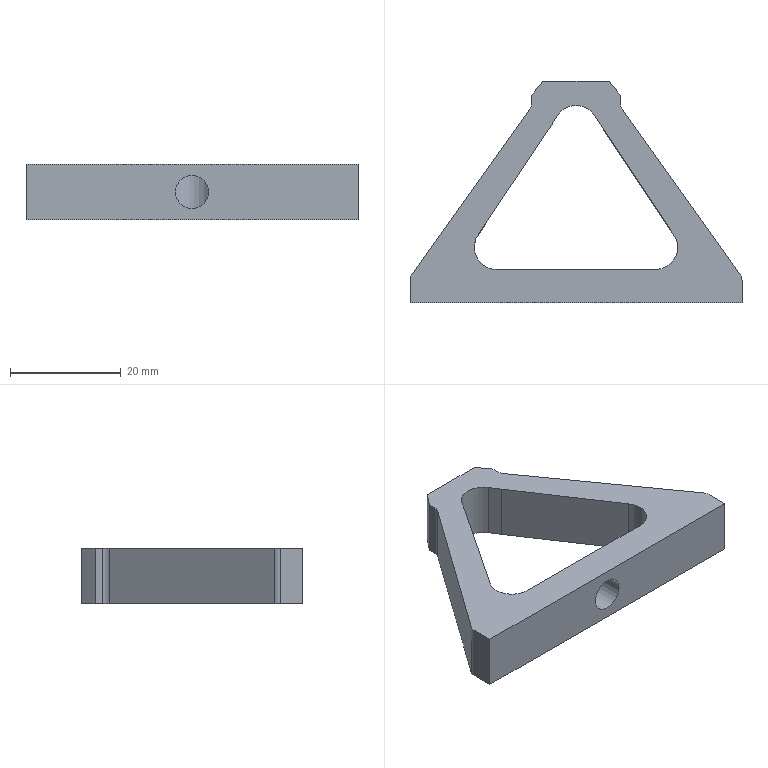Part | SolidWorks | features Extrusion 1, ICE 1 | 1 solid | 27 faces | box 60 x 40 x 10 mm | volume 8175 mm3 | plane 17 | cylinder 10 | commonest cylinder face diameters 4 x4 8 x4 6 x2
STEP:
#1=CARTESIAN_POINT('',(-3.485,-13.953,5.));
#2=VERTEX_POINT('',#1);
#3=CARTESIAN_POINT('',(-9.485,-13.953,5.));
#4=VERTEX_POINT('',#3);
#5=CARTESIAN_POINT('',(-6.485,-13.953,5.));
#6=DIRECTION('',(0.,1.,0.));
#7=DIRECTION('',(-1.,0.,0.));
#8=AXIS2_PLACEMENT_3D('',#5,#6,#7);
#9=CIRCLE('',#8,3.);
#10=EDGE_CURVE('',#2,#4,#9,.T.);
#11=ORIENTED_EDGE('',*,*,#10,.T.);
#12=CARTESIAN_POINT('',(-9.485,-19.953,5.));
#13=VERTEX_POINT('',#12);
#14=CARTESIAN_POINT('',(-9.485,-9.953,5.));
#15=DIRECTION('',(0.,-1.,0.));
#16=VECTOR('',#15,1000.);
#17=LINE('',#14,#16);
#18=EDGE_CURVE('',#4,#13,#17,.T.);
#19=ORIENTED_EDGE('',*,*,#18,.T.);
#20=CARTESIAN_POINT('',(-3.485,-19.953,5.));
#21=VERTEX_POINT('',#20);
#22=CARTESIAN_POINT('',(-6.485,-19.953,5.));
#23=DIRECTION('',(0.,-1.,0.));
#24=DIRECTION('',(1.,0.,0.));
#25=AXIS2_PLACEMENT_3D('',#22,#23,#24);
#26=CIRCLE('',#25,3.);
#27=EDGE_CURVE('',#13,#21,#26,.T.);
#28=ORIENTED_EDGE('',*,*,#27,.T.);
#29=CARTESIAN_POINT('',(-3.485,-9.953,5.));
#30=DIRECTION('',(0.,-1.,0.));
#31=VECTOR('',#30,1000.);
#32=LINE('',#29,#31);
#33=EDGE_CURVE('',#2,#21,#32,.T.);
#34=ORIENTED_EDGE('',*,*,#33,.F.);
#35=EDGE_LOOP('',(#11,#19,#28,#34));
#36=FACE_OUTER_BOUND('',#35,.T.);
#37=CARTESIAN_POINT('',(-6.485,-9.953,5.));
#38=DIRECTION('',(0.,-1.,0.));
#39=DIRECTION('',(1.,0.,0.));
#40=AXIS2_PLACEMENT_3D('',#37,#38,#39);
#41=CYLINDRICAL_SURFACE('',#40,3.);
#42=ADVANCED_FACE('',(#36),#41,.F.);
#43=CARTESIAN_POINT('',(-24.192,-7.733,10.));
#44=VERTEX_POINT('',#43);
#45=CARTESIAN_POINT('',(-24.865,-9.953,10.));
#46=VERTEX_POINT('',#45);
#47=CARTESIAN_POINT('',(-20.865,-9.953,10.));
#48=DIRECTION('',(0.,0.,1.));
#49=DIRECTION('',(-1.,0.,0.));
#50=AXIS2_PLACEMENT_3D('',#47,#48,#49);
#51=CIRCLE('',#50,4.);
#52=EDGE_CURVE('',#44,#46,#51,.T.);
#53=ORIENTED_EDGE('',*,*,#52,.T.);
#54=CARTESIAN_POINT('',(-24.865,-9.953,0.));
#55=VERTEX_POINT('',#54);
#56=CARTESIAN_POINT('',(-24.865,-9.953,10.));
#57=DIRECTION('',(0.,0.,-1.));
#58=VECTOR('',#57,1000.);
#59=LINE('',#56,#58);
#60=EDGE_CURVE('',#46,#55,#59,.T.);
#61=ORIENTED_EDGE('',*,*,#60,.T.);
#62=CARTESIAN_POINT('',(-24.192,-7.733,0.));
#63=VERTEX_POINT('',#62);
#64=CARTESIAN_POINT('',(-20.865,-9.953,0.));
#65=DIRECTION('',(0.,0.,1.));
#66=DIRECTION('',(-1.,0.,0.));
#67=AXIS2_PLACEMENT_3D('',#64,#65,#66);
#68=CIRCLE('',#67,4.);
#69=EDGE_CURVE('',#63,#55,#68,.T.);
#70=ORIENTED_EDGE('',*,*,#69,.F.);
#71=CARTESIAN_POINT('',(-24.192,-7.733,10.));
#72=DIRECTION('',(0.,0.,-1.));
#73=VECTOR('',#72,1000.);
#74=LINE('',#71,#73);
#75=EDGE_CURVE('',#44,#63,#74,.T.);
#76=ORIENTED_EDGE('',*,*,#75,.F.);
#77=EDGE_LOOP('',(#53,#61,#70,#76));
#78=FACE_OUTER_BOUND('',#77,.T.);
#79=CARTESIAN_POINT('',(-20.865,-9.953,10.));
#80=DIRECTION('',(0.,0.,-1.));
#81=DIRECTION('',(-1.,0.,0.));
#82=AXIS2_PLACEMENT_3D('',#79,#80,#81);
#83=CYLINDRICAL_SURFACE('',#82,4.);
#84=ADVANCED_FACE('',(#78),#83,.F.);
#85=CARTESIAN_POINT('',(-36.485,-15.953,10.));
#86=VERTEX_POINT('',#85);
#87=CARTESIAN_POINT('',(-36.485,-19.953,10.));
#88=VERTEX_POINT('',#87);
#89=CARTESIAN_POINT('',(-36.485,-19.953,10.));
#90=DIRECTION('',(0.,-1.,0.));
#91=VECTOR('',#90,1000.);
#92=LINE('',#89,#91);
#93=EDGE_CURVE('',#86,#88,#92,.T.);
#94=ORIENTED_EDGE('',*,*,#93,.T.);
#95=CARTESIAN_POINT('',(23.515,-19.953,10.));
#96=VERTEX_POINT('',#95);
#97=CARTESIAN_POINT('',(-36.485,-19.953,10.));
#98=DIRECTION('',(1.,0.,0.));
#99=VECTOR('',#98,1000.);
#100=LINE('',#97,#99);
#101=EDGE_CURVE('',#88,#96,#100,.T.);
#102=ORIENTED_EDGE('',*,*,#101,.T.);
#103=CARTESIAN_POINT('',(23.515,-15.953,10.));
#104=VERTEX_POINT('',#103);
#105=CARTESIAN_POINT('',(23.515,-19.953,10.));
#106=DIRECTION('',(0.,1.,0.));
#107=VECTOR('',#106,1000.);
#108=LINE('',#105,#107);
#109=EDGE_CURVE('',#96,#104,#108,.T.);
#110=ORIENTED_EDGE('',*,*,#109,.T.);
#111=CARTESIAN_POINT('',(23.179,-14.843,10.));
#112=VERTEX_POINT('',#111);
#113=CARTESIAN_POINT('',(21.515,-15.953,10.));
#114=DIRECTION('',(0.,0.,1.));
#115=DIRECTION('',(1.,0.,0.));
#116=AXIS2_PLACEMENT_3D('',#113,#114,#115);
#117=CIRCLE('',#116,2.);
#118=EDGE_CURVE('',#104,#112,#117,.T.);
#119=ORIENTED_EDGE('',*,*,#118,.T.);
#120=CARTESIAN_POINT('',(1.887,15.02,10.));
#121=VERTEX_POINT('',#120);
#122=CARTESIAN_POINT('',(1.887,15.02,10.));
#123=DIRECTION('',(-0.5805,0.8142,0.));
#124=VECTOR('',#123,1000.);
#125=LINE('',#122,#124);
#126=EDGE_CURVE('',#112,#121,#125,.T.);
#127=ORIENTED_EDGE('',*,*,#126,.T.);
#128=CARTESIAN_POINT('',(1.515,16.181,10.));
#129=VERTEX_POINT('',#128);
#130=CARTESIAN_POINT('',(3.515,16.181,10.));
#131=DIRECTION('',(0.,0.,-1.));
#132=DIRECTION('',(-1.,0.,0.));
#133=AXIS2_PLACEMENT_3D('',#130,#131,#132);
#134=CIRCLE('',#133,2.);
#135=EDGE_CURVE('',#121,#129,#134,.T.);
#136=ORIENTED_EDGE('',*,*,#135,.T.);
#137=CARTESIAN_POINT('',(1.515,17.541,10.));
#138=VERTEX_POINT('',#137);
#139=CARTESIAN_POINT('',(1.515,16.181,10.));
#140=DIRECTION('',(0.,1.,0.));
#141=VECTOR('',#140,1000.);
#142=LINE('',#139,#141);
#143=EDGE_CURVE('',#129,#138,#142,.T.);
#144=ORIENTED_EDGE('',*,*,#143,.T.);
#145=CARTESIAN_POINT('',(-0.4847,20.047,10.));
#146=VERTEX_POINT('',#145);
#147=CARTESIAN_POINT('',(1.515,17.541,10.));
#148=DIRECTION('',(-0.6238,0.7816,0.));
#149=VECTOR('',#148,1000.);
#150=LINE('',#147,#149);
#151=EDGE_CURVE('',#138,#146,#150,.T.);
#152=ORIENTED_EDGE('',*,*,#151,.T.);
#153=CARTESIAN_POINT('',(-12.485,20.047,10.));
#154=VERTEX_POINT('',#153);
#155=CARTESIAN_POINT('',(-12.485,20.047,10.));
#156=DIRECTION('',(-1.,0.,0.));
#157=VECTOR('',#156,1000.);
#158=LINE('',#155,#157);
#159=EDGE_CURVE('',#146,#154,#158,.T.);
#160=ORIENTED_EDGE('',*,*,#159,.T.);
#161=CARTESIAN_POINT('',(-14.485,17.541,10.));
#162=VERTEX_POINT('',#161);
#163=CARTESIAN_POINT('',(-14.485,17.541,10.));
#164=DIRECTION('',(-0.6238,-0.7816,0.));
#165=VECTOR('',#164,1000.);
#166=LINE('',#163,#165);
#167=EDGE_CURVE('',#154,#162,#166,.T.);
#168=ORIENTED_EDGE('',*,*,#167,.T.);
#169=CARTESIAN_POINT('',(-14.485,16.181,10.));
#170=VERTEX_POINT('',#169);
#171=CARTESIAN_POINT('',(-14.485,16.181,10.));
#172=DIRECTION('',(0.,-1.,0.));
#173=VECTOR('',#172,1000.);
#174=LINE('',#171,#173);
#175=EDGE_CURVE('',#162,#170,#174,.T.);
#176=ORIENTED_EDGE('',*,*,#175,.T.);
#177=CARTESIAN_POINT('',(-14.856,15.02,10.));
#178=VERTEX_POINT('',#177);
#179=CARTESIAN_POINT('',(-16.485,16.181,10.));
#180=DIRECTION('',(0.,0.,-1.));
#181=DIRECTION('',(1.,0.,0.));
#182=AXIS2_PLACEMENT_3D('',#179,#180,#181);
#183=CIRCLE('',#182,2.);
#184=EDGE_CURVE('',#170,#178,#183,.T.);
#185=ORIENTED_EDGE('',*,*,#184,.T.);
#186=CARTESIAN_POINT('',(-36.148,-14.843,10.));
#187=VERTEX_POINT('',#186);
#188=CARTESIAN_POINT('',(-36.148,-14.843,10.));
#189=DIRECTION('',(-0.5805,-0.8142,0.));
#190=VECTOR('',#189,1000.);
#191=LINE('',#188,#190);
#192=EDGE_CURVE('',#178,#187,#191,.T.);
#193=ORIENTED_EDGE('',*,*,#192,.T.);
#194=CARTESIAN_POINT('',(-34.485,-15.953,10.));
#195=DIRECTION('',(0.,0.,1.));
#196=DIRECTION('',(-1.,0.,0.));
#197=AXIS2_PLACEMENT_3D('',#194,#195,#196);
#198=CIRCLE('',#197,2.);
#199=EDGE_CURVE('',#187,#86,#198,.T.);
#200=ORIENTED_EDGE('',*,*,#199,.T.);
#201=EDGE_LOOP('',(#94,#102,#110,#119,#127,#136,#144,#152,#160,#168,#176,#185,#193,#200));
#202=FACE_OUTER_BOUND('',#201,.T.);
#203=CARTESIAN_POINT('',(-9.853,13.848,10.));
#204=VERTEX_POINT('',#203);
#205=CARTESIAN_POINT('',(-11.182,11.768,10.));
#206=VERTEX_POINT('',#205);
#207=CARTESIAN_POINT('',(-11.182,11.768,10.));
#208=DIRECTION('',(-0.5383,-0.8427,0.));
#209=VECTOR('',#208,1000.);
#210=LINE('',#207,#209);
#211=EDGE_CURVE('',#204,#206,#210,.T.);
#212=ORIENTED_EDGE('',*,*,#211,.F.);
#213=CARTESIAN_POINT('',(-3.113,13.85,10.));
#214=VERTEX_POINT('',#213);
#215=CARTESIAN_POINT('',(-6.482,11.695,10.));
#216=DIRECTION('',(0.,0.,1.));
#217=DIRECTION('',(1.,0.,0.));
#218=AXIS2_PLACEMENT_3D('',#215,#216,#217);
#219=CIRCLE('',#218,4.);
#220=EDGE_CURVE('',#214,#204,#219,.T.);
#221=ORIENTED_EDGE('',*,*,#220,.F.);
#222=CARTESIAN_POINT('',(-1.803,11.803,10.));
#223=VERTEX_POINT('',#222);
#224=CARTESIAN_POINT('',(-1.803,11.803,10.));
#225=DIRECTION('',(-0.5389,0.8424,0.));
#226=VECTOR('',#225,1000.);
#227=LINE('',#224,#226);
#228=EDGE_CURVE('',#223,#214,#227,.T.);
#229=ORIENTED_EDGE('',*,*,#228,.F.);
#230=CARTESIAN_POINT('',(11.226,-7.734,10.));
#231=VERTEX_POINT('',#230);
#232=CARTESIAN_POINT('',(-1.803,11.803,10.));
#233=DIRECTION('',(-0.5548,0.832,0.));
#234=VECTOR('',#233,1000.);
#235=LINE('',#232,#234);
#236=EDGE_CURVE('',#231,#223,#235,.T.);
#237=ORIENTED_EDGE('',*,*,#236,.F.);
#238=CARTESIAN_POINT('',(7.898,-13.953,10.));
#239=VERTEX_POINT('',#238);
#240=CARTESIAN_POINT('',(7.898,-9.953,10.));
#241=DIRECTION('',(0.,0.,1.));
#242=DIRECTION('',(-1.,0.,0.));
#243=AXIS2_PLACEMENT_3D('',#240,#241,#242);
#244=CIRCLE('',#243,4.);
#245=EDGE_CURVE('',#239,#231,#244,.T.);
#246=ORIENTED_EDGE('',*,*,#245,.F.);
#247=CARTESIAN_POINT('',(-20.865,-13.953,10.));
#248=VERTEX_POINT('',#247);
#249=CARTESIAN_POINT('',(-20.865,-13.953,10.));
#250=DIRECTION('',(1.,0.,0.));
#251=VECTOR('',#250,1000.);
#252=LINE('',#249,#251);
#253=EDGE_CURVE('',#248,#239,#252,.T.);
#254=ORIENTED_EDGE('',*,*,#253,.F.);
#255=CARTESIAN_POINT('',(-20.865,-9.953,10.));
#256=DIRECTION('',(0.,0.,1.));
#257=DIRECTION('',(-1.,0.,0.));
#258=AXIS2_PLACEMENT_3D('',#255,#256,#257);
#259=CIRCLE('',#258,4.);
#260=EDGE_CURVE('',#46,#248,#259,.T.);
#261=ORIENTED_EDGE('',*,*,#260,.F.);
#262=ORIENTED_EDGE('',*,*,#52,.F.);
#263=CARTESIAN_POINT('',(-24.192,-7.733,10.));
#264=DIRECTION('',(-0.555,-0.8319,0.));
#265=VECTOR('',#264,1000.);
#266=LINE('',#263,#265);
#267=EDGE_CURVE('',#206,#44,#266,.T.);
#268=ORIENTED_EDGE('',*,*,#267,.F.);
#269=EDGE_LOOP('',(#212,#221,#229,#237,#246,#254,#261,#262,#268));
#270=FACE_BOUND('',#269,.T.);
#271=CARTESIAN_POINT('',(-34.485,-15.953,10.));
#272=DIRECTION('',(0.,0.,-1.));
#273=DIRECTION('',(-1.,0.,0.));
#274=AXIS2_PLACEMENT_3D('',#271,#272,#273);
#275=PLANE('',#274);
#276=ADVANCED_FACE('',(#202,#270),#275,.F.);
#277=CARTESIAN_POINT('',(-36.485,-15.953,0.));
#278=VERTEX_POINT('',#277);
#279=CARTESIAN_POINT('',(-36.485,-19.953,0.));
#280=VERTEX_POINT('',#279);
#281=CARTESIAN_POINT('',(-36.485,-19.953,0.));
#282=DIRECTION('',(0.,-1.,0.));
#283=VECTOR('',#282,1000.);
#284=LINE('',#281,#283);
#285=EDGE_CURVE('',#278,#280,#284,.T.);
#286=ORIENTED_EDGE('',*,*,#285,.F.);
#287=CARTESIAN_POINT('',(-36.148,-14.843,0.));
#288=VERTEX_POINT('',#287);
#289=CARTESIAN_POINT('',(-34.485,-15.953,0.));
#290=DIRECTION('',(0.,0.,1.));
#291=DIRECTION('',(-1.,0.,0.));
#292=AXIS2_PLACEMENT_3D('',#289,#290,#291);
#293=CIRCLE('',#292,2.);
#294=EDGE_CURVE('',#288,#278,#293,.T.);
#295=ORIENTED_EDGE('',*,*,#294,.F.);
#296=CARTESIAN_POINT('',(-14.856,15.02,0.));
#297=VERTEX_POINT('',#296);
#298=CARTESIAN_POINT('',(-36.148,-14.843,0.));
#299=DIRECTION('',(-0.5805,-0.8142,0.));
#300=VECTOR('',#299,1000.);
#301=LINE('',#298,#300);
#302=EDGE_CURVE('',#297,#288,#301,.T.);
#303=ORIENTED_EDGE('',*,*,#302,.F.);
#304=CARTESIAN_POINT('',(-14.485,16.181,0.));
#305=VERTEX_POINT('',#304);
#306=CARTESIAN_POINT('',(-16.485,16.181,0.));
#307=DIRECTION('',(0.,0.,-1.));
#308=DIRECTION('',(1.,0.,0.));
#309=AXIS2_PLACEMENT_3D('',#306,#307,#308);
#310=CIRCLE('',#309,2.);
#311=EDGE_CURVE('',#305,#297,#310,.T.);
#312=ORIENTED_EDGE('',*,*,#311,.F.);
#313=CARTESIAN_POINT('',(-14.485,17.541,0.));
#314=VERTEX_POINT('',#313);
#315=CARTESIAN_POINT('',(-14.485,16.181,0.));
#316=DIRECTION('',(0.,-1.,0.));
#317=VECTOR('',#316,1000.);
#318=LINE('',#315,#317);
#319=EDGE_CURVE('',#314,#305,#318,.T.);
#320=ORIENTED_EDGE('',*,*,#319,.F.);
#321=CARTESIAN_POINT('',(-12.485,20.047,0.));
#322=VERTEX_POINT('',#321);
#323=CARTESIAN_POINT('',(-14.485,17.541,0.));
#324=DIRECTION('',(-0.6238,-0.7816,0.));
#325=VECTOR('',#324,1000.);
#326=LINE('',#323,#325);
#327=EDGE_CURVE('',#322,#314,#326,.T.);
#328=ORIENTED_EDGE('',*,*,#327,.F.);
#329=CARTESIAN_POINT('',(-0.4847,20.047,0.));
#330=VERTEX_POINT('',#329);
#331=CARTESIAN_POINT('',(-12.485,20.047,0.));
#332=DIRECTION('',(-1.,0.,0.));
#333=VECTOR('',#332,1000.);
#334=LINE('',#331,#333);
#335=EDGE_CURVE('',#330,#322,#334,.T.);
#336=ORIENTED_EDGE('',*,*,#335,.F.);
#337=CARTESIAN_POINT('',(1.515,17.541,0.));
#338=VERTEX_POINT('',#337);
#339=CARTESIAN_POINT('',(1.515,17.541,0.));
#340=DIRECTION('',(-0.6238,0.7816,0.));
#341=VECTOR('',#340,1000.);
#342=LINE('',#339,#341);
#343=EDGE_CURVE('',#338,#330,#342,.T.);
#344=ORIENTED_EDGE('',*,*,#343,.F.);
#345=CARTESIAN_POINT('',(1.515,16.181,0.));
#346=VERTEX_POINT('',#345);
#347=CARTESIAN_POINT('',(1.515,16.181,0.));
#348=DIRECTION('',(0.,1.,0.));
#349=VECTOR('',#348,1000.);
#350=LINE('',#347,#349);
#351=EDGE_CURVE('',#346,#338,#350,.T.);
#352=ORIENTED_EDGE('',*,*,#351,.F.);
#353=CARTESIAN_POINT('',(1.887,15.02,0.));
#354=VERTEX_POINT('',#353);
#355=CARTESIAN_POINT('',(3.515,16.181,0.));
#356=DIRECTION('',(0.,0.,-1.));
#357=DIRECTION('',(-1.,0.,0.));
#358=AXIS2_PLACEMENT_3D('',#355,#356,#357);
#359=CIRCLE('',#358,2.);
#360=EDGE_CURVE('',#354,#346,#359,.T.);
#361=ORIENTED_EDGE('',*,*,#360,.F.);
#362=CARTESIAN_POINT('',(23.179,-14.843,0.));
#363=VERTEX_POINT('',#362);
#364=CARTESIAN_POINT('',(1.887,15.02,0.));
#365=DIRECTION('',(-0.5805,0.8142,0.));
#366=VECTOR('',#365,1000.);
#367=LINE('',#364,#366);
#368=EDGE_CURVE('',#363,#354,#367,.T.);
#369=ORIENTED_EDGE('',*,*,#368,.F.);
#370=CARTESIAN_POINT('',(23.515,-15.953,0.));
#371=VERTEX_POINT('',#370);
#372=CARTESIAN_POINT('',(21.515,-15.953,0.));
#373=DIRECTION('',(0.,0.,1.));
#374=DIRECTION('',(1.,0.,0.));
#375=AXIS2_PLACEMENT_3D('',#372,#373,#374);
#376=CIRCLE('',#375,2.);
#377=EDGE_CURVE('',#371,#363,#376,.T.);
#378=ORIENTED_EDGE('',*,*,#377,.F.);
#379=CARTESIAN_POINT('',(23.515,-19.953,0.));
#380=VERTEX_POINT('',#379);
#381=CARTESIAN_POINT('',(23.515,-19.953,0.));
#382=DIRECTION('',(0.,1.,0.));
#383=VECTOR('',#382,1000.);
#384=LINE('',#381,#383);
#385=EDGE_CURVE('',#380,#371,#384,.T.);
#386=ORIENTED_EDGE('',*,*,#385,.F.);
#387=CARTESIAN_POINT('',(-36.485,-19.953,0.));
#388=DIRECTION('',(1.,0.,0.));
#389=VECTOR('',#388,1000.);
#390=LINE('',#387,#389);
#391=EDGE_CURVE('',#280,#380,#390,.T.);
#392=ORIENTED_EDGE('',*,*,#391,.F.);
#393=EDGE_LOOP('',(#286,#295,#303,#312,#320,#328,#336,#344,#352,#361,#369,#378,#386,#392));
#394=FACE_OUTER_BOUND('',#393,.T.);
#395=CARTESIAN_POINT('',(-3.113,13.85,0.));
#396=VERTEX_POINT('',#395);
#397=CARTESIAN_POINT('',(-9.853,13.848,0.));
#398=VERTEX_POINT('',#397);
#399=CARTESIAN_POINT('',(-6.482,11.695,0.));
#400=DIRECTION('',(0.,0.,1.));
#401=DIRECTION('',(1.,0.,0.));
#402=AXIS2_PLACEMENT_3D('',#399,#400,#401);
#403=CIRCLE('',#402,4.);
#404=EDGE_CURVE('',#396,#398,#403,.T.);
#405=ORIENTED_EDGE('',*,*,#404,.T.);
#406=CARTESIAN_POINT('',(-11.182,11.768,0.));
#407=VERTEX_POINT('',#406);
#408=CARTESIAN_POINT('',(-11.182,11.768,0.));
#409=DIRECTION('',(-0.5383,-0.8427,0.));
#410=VECTOR('',#409,1000.);
#411=LINE('',#408,#410);
#412=EDGE_CURVE('',#398,#407,#411,.T.);
#413=ORIENTED_EDGE('',*,*,#412,.T.);
#414=CARTESIAN_POINT('',(-24.192,-7.733,0.));
#415=DIRECTION('',(-0.555,-0.8319,0.));
#416=VECTOR('',#415,1000.);
#417=LINE('',#414,#416);
#418=EDGE_CURVE('',#407,#63,#417,.T.);
#419=ORIENTED_EDGE('',*,*,#418,.T.);
#420=ORIENTED_EDGE('',*,*,#69,.T.);
#421=CARTESIAN_POINT('',(-20.865,-13.953,0.));
#422=VERTEX_POINT('',#421);
#423=CARTESIAN_POINT('',(-20.865,-9.953,0.));
#424=DIRECTION('',(0.,0.,1.));
#425=DIRECTION('',(-1.,0.,0.));
#426=AXIS2_PLACEMENT_3D('',#423,#424,#425);
#427=CIRCLE('',#426,4.);
#428=EDGE_CURVE('',#55,#422,#427,.T.);
#429=ORIENTED_EDGE('',*,*,#428,.T.);
#430=CARTESIAN_POINT('',(7.898,-13.953,0.));
#431=VERTEX_POINT('',#430);
#432=CARTESIAN_POINT('',(-20.865,-13.953,0.));
#433=DIRECTION('',(1.,0.,0.));
#434=VECTOR('',#433,1000.);
#435=LINE('',#432,#434);
#436=EDGE_CURVE('',#422,#431,#435,.T.);
#437=ORIENTED_EDGE('',*,*,#436,.T.);
#438=CARTESIAN_POINT('',(11.226,-7.734,0.));
#439=VERTEX_POINT('',#438);
#440=CARTESIAN_POINT('',(7.898,-9.953,0.));
#441=DIRECTION('',(0.,0.,1.));
#442=DIRECTION('',(-1.,0.,0.));
#443=AXIS2_PLACEMENT_3D('',#440,#441,#442);
#444=CIRCLE('',#443,4.);
#445=EDGE_CURVE('',#431,#439,#444,.T.);
#446=ORIENTED_EDGE('',*,*,#445,.T.);
#447=CARTESIAN_POINT('',(-1.803,11.803,0.));
#448=VERTEX_POINT('',#447);
#449=CARTESIAN_POINT('',(-1.803,11.803,0.));
#450=DIRECTION('',(-0.5548,0.832,0.));
#451=VECTOR('',#450,1000.);
#452=LINE('',#449,#451);
#453=EDGE_CURVE('',#439,#448,#452,.T.);
#454=ORIENTED_EDGE('',*,*,#453,.T.);
#455=CARTESIAN_POINT('',(-1.803,11.803,0.));
#456=DIRECTION('',(-0.5389,0.8424,0.));
#457=VECTOR('',#456,1000.);
#458=LINE('',#455,#457);
#459=EDGE_CURVE('',#448,#396,#458,.T.);
#460=ORIENTED_EDGE('',*,*,#459,.T.);
#461=EDGE_LOOP('',(#405,#413,#419,#420,#429,#437,#446,#454,#460));
#462=FACE_BOUND('',#461,.T.);
#463=CARTESIAN_POINT('',(-34.485,-15.953,0.));
#464=DIRECTION('',(0.,0.,-1.));
#465=DIRECTION('',(-1.,0.,0.));
#466=AXIS2_PLACEMENT_3D('',#463,#464,#465);
#467=PLANE('',#466);
#468=ADVANCED_FACE('',(#394,#462),#467,.T.);
#469=ORIENTED_EDGE('',*,*,#285,.T.);
#470=CARTESIAN_POINT('',(-36.485,-19.953,10.));
#471=DIRECTION('',(0.,0.,-1.));
#472=VECTOR('',#471,1000.);
#473=LINE('',#470,#472);
#474=EDGE_CURVE('',#88,#280,#473,.T.);
#475=ORIENTED_EDGE('',*,*,#474,.F.);
#476=ORIENTED_EDGE('',*,*,#93,.F.);
#477=CARTESIAN_POINT('',(-36.485,-15.953,10.));
#478=DIRECTION('',(0.,0.,-1.));
#479=VECTOR('',#478,1000.);
#480=LINE('',#477,#479);
#481=EDGE_CURVE('',#86,#278,#480,.T.);
#482=ORIENTED_EDGE('',*,*,#481,.T.);
#483=EDGE_LOOP('',(#469,#475,#476,#482));
#484=FACE_OUTER_BOUND('',#483,.T.);
#485=CARTESIAN_POINT('',(-36.485,-19.953,10.));
#486=DIRECTION('',(1.,0.,0.));
#487=DIRECTION('',(0.,0.,-1.));
#488=AXIS2_PLACEMENT_3D('',#485,#486,#487);
#489=PLANE('',#488);
#490=ADVANCED_FACE('',(#484),#489,.F.);
#491=CARTESIAN_POINT('',(-6.485,-19.953,5.));
#492=DIRECTION('',(0.,-1.,0.));
#493=DIRECTION('',(1.,0.,0.));
#494=AXIS2_PLACEMENT_3D('',#491,#492,#493);
#495=CIRCLE('',#494,3.);
#496=EDGE_CURVE('',#21,#13,#495,.T.);
#497=ORIENTED_EDGE('',*,*,#496,.F.);
#498=ORIENTED_EDGE('',*,*,#27,.F.);
#499=EDGE_LOOP('',(#497,#498));
#500=FACE_BOUND('',#499,.T.);
#501=ORIENTED_EDGE('',*,*,#391,.T.);
#502=CARTESIAN_POINT('',(23.515,-19.953,10.));
#503=DIRECTION('',(0.,0.,-1.));
#504=VECTOR('',#503,1000.);
#505=LINE('',#502,#504);
#506=EDGE_CURVE('',#96,#380,#505,.T.);
#507=ORIENTED_EDGE('',*,*,#506,.F.);
#508=ORIENTED_EDGE('',*,*,#101,.F.);
#509=ORIENTED_EDGE('',*,*,#474,.T.);
#510=EDGE_LOOP('',(#501,#507,#508,#509));
#511=FACE_OUTER_BOUND('',#510,.T.);
#512=CARTESIAN_POINT('',(-36.485,-19.953,10.));
#513=DIRECTION('',(0.,1.,0.));
#514=DIRECTION('',(-1.,0.,0.));
#515=AXIS2_PLACEMENT_3D('',#512,#513,#514);
#516=PLANE('',#515);
#517=ADVANCED_FACE('',(#500,#511),#516,.F.);
#518=ORIENTED_EDGE('',*,*,#385,.T.);
#519=CARTESIAN_POINT('',(23.515,-15.953,10.));
#520=DIRECTION('',(0.,0.,-1.));
#521=VECTOR('',#520,1000.);
#522=LINE('',#519,#521);
#523=EDGE_CURVE('',#104,#371,#522,.T.);
#524=ORIENTED_EDGE('',*,*,#523,.F.);
#525=ORIENTED_EDGE('',*,*,#109,.F.);
#526=ORIENTED_EDGE('',*,*,#506,.T.);
#527=EDGE_LOOP('',(#518,#524,#525,#526));
#528=FACE_OUTER_BOUND('',#527,.T.);
#529=CARTESIAN_POINT('',(23.515,-19.953,10.));
#530=DIRECTION('',(-1.,0.,0.));
#531=DIRECTION('',(0.,0.,1.));
#532=AXIS2_PLACEMENT_3D('',#529,#530,#531);
#533=PLANE('',#532);
#534=ADVANCED_FACE('',(#528),#533,.F.);
#535=ORIENTED_EDGE('',*,*,#377,.T.);
#536=CARTESIAN_POINT('',(23.179,-14.843,10.));
#537=DIRECTION('',(0.,0.,-1.));
#538=VECTOR('',#537,1000.);
#539=LINE('',#536,#538);
#540=EDGE_CURVE('',#112,#363,#539,.T.);
#541=ORIENTED_EDGE('',*,*,#540,.F.);
#542=ORIENTED_EDGE('',*,*,#118,.F.);
#543=ORIENTED_EDGE('',*,*,#523,.T.);
#544=EDGE_LOOP('',(#535,#541,#542,#543));
#545=FACE_OUTER_BOUND('',#544,.T.);
#546=CARTESIAN_POINT('',(21.515,-15.953,10.));
#547=DIRECTION('',(0.,0.,-1.));
#548=DIRECTION('',(-1.,0.,0.));
#549=AXIS2_PLACEMENT_3D('',#546,#547,#548);
#550=CYLINDRICAL_SURFACE('',#549,2.);
#551=ADVANCED_FACE('',(#545),#550,.T.);
#552=ORIENTED_EDGE('',*,*,#368,.T.);
#553=CARTESIAN_POINT('',(1.887,15.02,10.));
#554=DIRECTION('',(0.,0.,-1.));
#555=VECTOR('',#554,1000.);
#556=LINE('',#553,#555);
#557=EDGE_CURVE('',#121,#354,#556,.T.);
#558=ORIENTED_EDGE('',*,*,#557,.F.);
#559=ORIENTED_EDGE('',*,*,#126,.F.);
#560=ORIENTED_EDGE('',*,*,#540,.T.);
#561=EDGE_LOOP('',(#552,#558,#559,#560));
#562=FACE_OUTER_BOUND('',#561,.T.);
#563=CARTESIAN_POINT('',(1.887,15.02,10.));
#564=DIRECTION('',(-0.8142,-0.5805,0.));
#565=DIRECTION('',(0.5805,-0.8142,0.));
#566=AXIS2_PLACEMENT_3D('',#563,#564,#565);
#567=PLANE('',#566);
#568=ADVANCED_FACE('',(#562),#567,.F.);
#569=ORIENTED_EDGE('',*,*,#360,.T.);
#570=CARTESIAN_POINT('',(1.515,16.181,10.));
#571=DIRECTION('',(0.,0.,-1.));
#572=VECTOR('',#571,1000.);
#573=LINE('',#570,#572);
#574=EDGE_CURVE('',#129,#346,#573,.T.);
#575=ORIENTED_EDGE('',*,*,#574,.F.);
#576=ORIENTED_EDGE('',*,*,#135,.F.);
#577=ORIENTED_EDGE('',*,*,#557,.T.);
#578=EDGE_LOOP('',(#569,#575,#576,#577));
#579=FACE_OUTER_BOUND('',#578,.T.);
#580=CARTESIAN_POINT('',(3.515,16.181,10.));
#581=DIRECTION('',(0.,0.,-1.));
#582=DIRECTION('',(-1.,0.,0.));
#583=AXIS2_PLACEMENT_3D('',#580,#581,#582);
#584=CYLINDRICAL_SURFACE('',#583,2.);
#585=ADVANCED_FACE('',(#579),#584,.F.);
#586=ORIENTED_EDGE('',*,*,#351,.T.);
#587=CARTESIAN_POINT('',(1.515,17.541,10.));
#588=DIRECTION('',(0.,0.,-1.));
#589=VECTOR('',#588,1000.);
#590=LINE('',#587,#589);
#591=EDGE_CURVE('',#138,#338,#590,.T.);
#592=ORIENTED_EDGE('',*,*,#591,.F.);
#593=ORIENTED_EDGE('',*,*,#143,.F.);
#594=ORIENTED_EDGE('',*,*,#574,.T.);
#595=EDGE_LOOP('',(#586,#592,#593,#594));
#596=FACE_OUTER_BOUND('',#595,.T.);
#597=CARTESIAN_POINT('',(1.515,16.181,10.));
#598=DIRECTION('',(-1.,0.,0.));
#599=DIRECTION('',(0.,0.,1.));
#600=AXIS2_PLACEMENT_3D('',#597,#598,#599);
#601=PLANE('',#600);
#602=ADVANCED_FACE('',(#596),#601,.F.);
#603=ORIENTED_EDGE('',*,*,#343,.T.);
#604=CARTESIAN_POINT('',(-0.4847,20.047,10.));
#605=DIRECTION('',(0.,0.,-1.));
#606=VECTOR('',#605,1000.);
#607=LINE('',#604,#606);
#608=EDGE_CURVE('',#146,#330,#607,.T.);
#609=ORIENTED_EDGE('',*,*,#608,.F.);
#610=ORIENTED_EDGE('',*,*,#151,.F.);
#611=ORIENTED_EDGE('',*,*,#591,.T.);
#612=EDGE_LOOP('',(#603,#609,#610,#611));
#613=FACE_OUTER_BOUND('',#612,.T.);
#614=CARTESIAN_POINT('',(1.515,17.541,10.));
#615=DIRECTION('',(-0.7816,-0.6238,0.));
#616=DIRECTION('',(0.6238,-0.7816,0.));
#617=AXIS2_PLACEMENT_3D('',#614,#615,#616);
#618=PLANE('',#617);
#619=ADVANCED_FACE('',(#613),#618,.F.);
#620=ORIENTED_EDGE('',*,*,#335,.T.);
#621=CARTESIAN_POINT('',(-12.485,20.047,10.));
#622=DIRECTION('',(0.,0.,-1.));
#623=VECTOR('',#622,1000.);
#624=LINE('',#621,#623);
#625=EDGE_CURVE('',#154,#322,#624,.T.);
#626=ORIENTED_EDGE('',*,*,#625,.F.);
#627=ORIENTED_EDGE('',*,*,#159,.F.);
#628=ORIENTED_EDGE('',*,*,#608,.T.);
#629=EDGE_LOOP('',(#620,#626,#627,#628));
#630=FACE_OUTER_BOUND('',#629,.T.);
#631=CARTESIAN_POINT('',(-12.485,20.047,10.));
#632=DIRECTION('',(0.,-1.,0.));
#633=DIRECTION('',(0.,0.,-1.));
#634=AXIS2_PLACEMENT_3D('',#631,#632,#633);
#635=PLANE('',#634);
#636=ADVANCED_FACE('',(#630),#635,.F.);
#637=ORIENTED_EDGE('',*,*,#327,.T.);
#638=CARTESIAN_POINT('',(-14.485,17.541,10.));
#639=DIRECTION('',(0.,0.,-1.));
#640=VECTOR('',#639,1000.);
#641=LINE('',#638,#640);
#642=EDGE_CURVE('',#162,#314,#641,.T.);
#643=ORIENTED_EDGE('',*,*,#642,.F.);
#644=ORIENTED_EDGE('',*,*,#167,.F.);
#645=ORIENTED_EDGE('',*,*,#625,.T.);
#646=EDGE_LOOP('',(#637,#643,#644,#645));
#647=FACE_OUTER_BOUND('',#646,.T.);
#648=CARTESIAN_POINT('',(-14.485,17.541,10.));
#649=DIRECTION('',(0.7816,-0.6238,0.));
#650=DIRECTION('',(0.6238,0.7816,0.));
#651=AXIS2_PLACEMENT_3D('',#648,#649,#650);
#652=PLANE('',#651);
#653=ADVANCED_FACE('',(#647),#652,.F.);
#654=ORIENTED_EDGE('',*,*,#319,.T.);
#655=CARTESIAN_POINT('',(-14.485,16.181,10.));
#656=DIRECTION('',(0.,0.,-1.));
#657=VECTOR('',#656,1000.);
#658=LINE('',#655,#657);
#659=EDGE_CURVE('',#170,#305,#658,.T.);
#660=ORIENTED_EDGE('',*,*,#659,.F.);
#661=ORIENTED_EDGE('',*,*,#175,.F.);
#662=ORIENTED_EDGE('',*,*,#642,.T.);
#663=EDGE_LOOP('',(#654,#660,#661,#662));
#664=FACE_OUTER_BOUND('',#663,.T.);
#665=CARTESIAN_POINT('',(-14.485,16.181,10.));
#666=DIRECTION('',(1.,0.,0.));
#667=DIRECTION('',(0.,0.,-1.));
#668=AXIS2_PLACEMENT_3D('',#665,#666,#667);
#669=PLANE('',#668);
#670=ADVANCED_FACE('',(#664),#669,.F.);
#671=ORIENTED_EDGE('',*,*,#311,.T.);
#672=CARTESIAN_POINT('',(-14.856,15.02,10.));
#673=DIRECTION('',(0.,0.,-1.));
#674=VECTOR('',#673,1000.);
#675=LINE('',#672,#674);
#676=EDGE_CURVE('',#178,#297,#675,.T.);
#677=ORIENTED_EDGE('',*,*,#676,.F.);
#678=ORIENTED_EDGE('',*,*,#184,.F.);
#679=ORIENTED_EDGE('',*,*,#659,.T.);
#680=EDGE_LOOP('',(#671,#677,#678,#679));
#681=FACE_OUTER_BOUND('',#680,.T.);
#682=CARTESIAN_POINT('',(-16.485,16.181,10.));
#683=DIRECTION('',(0.,0.,-1.));
#684=DIRECTION('',(-1.,0.,0.));
#685=AXIS2_PLACEMENT_3D('',#682,#683,#684);
#686=CYLINDRICAL_SURFACE('',#685,2.);
#687=ADVANCED_FACE('',(#681),#686,.F.);
#688=ORIENTED_EDGE('',*,*,#302,.T.);
#689=CARTESIAN_POINT('',(-36.148,-14.843,10.));
#690=DIRECTION('',(0.,0.,-1.));
#691=VECTOR('',#690,1000.);
#692=LINE('',#689,#691);
#693=EDGE_CURVE('',#187,#288,#692,.T.);
#694=ORIENTED_EDGE('',*,*,#693,.F.);
#695=ORIENTED_EDGE('',*,*,#192,.F.);
#696=ORIENTED_EDGE('',*,*,#676,.T.);
#697=EDGE_LOOP('',(#688,#694,#695,#696));
#698=FACE_OUTER_BOUND('',#697,.T.);
#699=CARTESIAN_POINT('',(-36.148,-14.843,10.));
#700=DIRECTION('',(0.8142,-0.5805,0.));
#701=DIRECTION('',(0.5805,0.8142,0.));
#702=AXIS2_PLACEMENT_3D('',#699,#700,#701);
#703=PLANE('',#702);
#704=ADVANCED_FACE('',(#698),#703,.F.);
#705=ORIENTED_EDGE('',*,*,#294,.T.);
#706=ORIENTED_EDGE('',*,*,#481,.F.);
#707=ORIENTED_EDGE('',*,*,#199,.F.);
#708=ORIENTED_EDGE('',*,*,#693,.T.);
#709=EDGE_LOOP('',(#705,#706,#707,#708));
#710=FACE_OUTER_BOUND('',#709,.T.);
#711=CARTESIAN_POINT('',(-34.485,-15.953,10.));
#712=DIRECTION('',(0.,0.,-1.));
#713=DIRECTION('',(-1.,0.,0.));
#714=AXIS2_PLACEMENT_3D('',#711,#712,#713);
#715=CYLINDRICAL_SURFACE('',#714,2.);
#716=ADVANCED_FACE('',(#710),#715,.T.);
#717=ORIENTED_EDGE('',*,*,#412,.F.);
#718=CARTESIAN_POINT('',(-9.853,13.848,10.));
#719=DIRECTION('',(0.,0.,-1.));
#720=VECTOR('',#719,1000.);
#721=LINE('',#718,#720);
#722=EDGE_CURVE('',#204,#398,#721,.T.);
#723=ORIENTED_EDGE('',*,*,#722,.F.);
#724=ORIENTED_EDGE('',*,*,#211,.T.);
#725=CARTESIAN_POINT('',(-11.182,11.768,10.));
#726=DIRECTION('',(0.,0.,-1.));
#727=VECTOR('',#726,1000.);
#728=LINE('',#725,#727);
#729=EDGE_CURVE('',#206,#407,#728,.T.);
#730=ORIENTED_EDGE('',*,*,#729,.T.);
#731=EDGE_LOOP('',(#717,#723,#724,#730));
#732=FACE_OUTER_BOUND('',#731,.T.);
#733=CARTESIAN_POINT('',(-11.182,11.768,10.));
#734=DIRECTION('',(0.8427,-0.5383,0.));
#735=DIRECTION('',(0.5383,0.8427,0.));
#736=AXIS2_PLACEMENT_3D('',#733,#734,#735);
#737=PLANE('',#736);
#738=ADVANCED_FACE('',(#732),#737,.T.);
#739=ORIENTED_EDGE('',*,*,#418,.F.);
#740=ORIENTED_EDGE('',*,*,#729,.F.);
#741=ORIENTED_EDGE('',*,*,#267,.T.);
#742=ORIENTED_EDGE('',*,*,#75,.T.);
#743=EDGE_LOOP('',(#739,#740,#741,#742));
#744=FACE_OUTER_BOUND('',#743,.T.);
#745=CARTESIAN_POINT('',(-24.192,-7.733,10.));
#746=DIRECTION('',(0.8319,-0.555,0.));
#747=DIRECTION('',(0.555,0.8319,0.));
#748=AXIS2_PLACEMENT_3D('',#745,#746,#747);
#749=PLANE('',#748);
#750=ADVANCED_FACE('',(#744),#749,.T.);
#751=ORIENTED_EDGE('',*,*,#60,.F.);
#752=ORIENTED_EDGE('',*,*,#260,.T.);
#753=CARTESIAN_POINT('',(-20.865,-13.953,10.));
#754=DIRECTION('',(0.,0.,-1.));
#755=VECTOR('',#754,1000.);
#756=LINE('',#753,#755);
#757=EDGE_CURVE('',#248,#422,#756,.T.);
#758=ORIENTED_EDGE('',*,*,#757,.T.);
#759=ORIENTED_EDGE('',*,*,#428,.F.);
#760=EDGE_LOOP('',(#751,#752,#758,#759));
#761=FACE_OUTER_BOUND('',#760,.T.);
#762=CARTESIAN_POINT('',(-20.865,-9.953,10.));
#763=DIRECTION('',(0.,0.,-1.));
#764=DIRECTION('',(-1.,0.,0.));
#765=AXIS2_PLACEMENT_3D('',#762,#763,#764);
#766=CYLINDRICAL_SURFACE('',#765,4.);
#767=ADVANCED_FACE('',(#761),#766,.F.);
#768=ORIENTED_EDGE('',*,*,#10,.F.);
#769=CARTESIAN_POINT('',(-6.485,-13.953,5.));
#770=DIRECTION('',(0.,1.,0.));
#771=DIRECTION('',(-1.,0.,0.));
#772=AXIS2_PLACEMENT_3D('',#769,#770,#771);
#773=CIRCLE('',#772,3.);
#774=EDGE_CURVE('',#4,#2,#773,.T.);
#775=ORIENTED_EDGE('',*,*,#774,.F.);
#776=EDGE_LOOP('',(#768,#775));
#777=FACE_BOUND('',#776,.T.);
#778=ORIENTED_EDGE('',*,*,#436,.F.);
#779=ORIENTED_EDGE('',*,*,#757,.F.);
#780=ORIENTED_EDGE('',*,*,#253,.T.);
#781=CARTESIAN_POINT('',(7.898,-13.953,10.));
#782=DIRECTION('',(0.,0.,-1.));
#783=VECTOR('',#782,1000.);
#784=LINE('',#781,#783);
#785=EDGE_CURVE('',#239,#431,#784,.T.);
#786=ORIENTED_EDGE('',*,*,#785,.T.);
#787=EDGE_LOOP('',(#778,#779,#780,#786));
#788=FACE_OUTER_BOUND('',#787,.T.);
#789=CARTESIAN_POINT('',(-20.865,-13.953,10.));
#790=DIRECTION('',(0.,1.,0.));
#791=DIRECTION('',(-1.,0.,0.));
#792=AXIS2_PLACEMENT_3D('',#789,#790,#791);
#793=PLANE('',#792);
#794=ADVANCED_FACE('',(#777,#788),#793,.T.);
#795=ORIENTED_EDGE('',*,*,#445,.F.);
#796=ORIENTED_EDGE('',*,*,#785,.F.);
#797=ORIENTED_EDGE('',*,*,#245,.T.);
#798=CARTESIAN_POINT('',(11.226,-7.734,10.));
#799=DIRECTION('',(0.,0.,-1.));
#800=VECTOR('',#799,1000.);
#801=LINE('',#798,#800);
#802=EDGE_CURVE('',#231,#439,#801,.T.);
#803=ORIENTED_EDGE('',*,*,#802,.T.);
#804=EDGE_LOOP('',(#795,#796,#797,#803));
#805=FACE_OUTER_BOUND('',#804,.T.);
#806=CARTESIAN_POINT('',(7.898,-9.953,10.));
#807=DIRECTION('',(0.,0.,-1.));
#808=DIRECTION('',(-1.,0.,0.));
#809=AXIS2_PLACEMENT_3D('',#806,#807,#808);
#810=CYLINDRICAL_SURFACE('',#809,4.);
#811=ADVANCED_FACE('',(#805),#810,.F.);
#812=ORIENTED_EDGE('',*,*,#453,.F.);
#813=ORIENTED_EDGE('',*,*,#802,.F.);
#814=ORIENTED_EDGE('',*,*,#236,.T.);
#815=CARTESIAN_POINT('',(-1.803,11.803,10.));
#816=DIRECTION('',(0.,0.,-1.));
#817=VECTOR('',#816,1000.);
#818=LINE('',#815,#817);
#819=EDGE_CURVE('',#223,#448,#818,.T.);
#820=ORIENTED_EDGE('',*,*,#819,.T.);
#821=EDGE_LOOP('',(#812,#813,#814,#820));
#822=FACE_OUTER_BOUND('',#821,.T.);
#823=CARTESIAN_POINT('',(-1.803,11.803,10.));
#824=DIRECTION('',(-0.832,-0.5548,0.));
#825=DIRECTION('',(0.5548,-0.832,0.));
#826=AXIS2_PLACEMENT_3D('',#823,#824,#825);
#827=PLANE('',#826);
#828=ADVANCED_FACE('',(#822),#827,.T.);
#829=ORIENTED_EDGE('',*,*,#459,.F.);
#830=ORIENTED_EDGE('',*,*,#819,.F.);
#831=ORIENTED_EDGE('',*,*,#228,.T.);
#832=CARTESIAN_POINT('',(-3.113,13.85,10.));
#833=DIRECTION('',(0.,0.,-1.));
#834=VECTOR('',#833,1000.);
#835=LINE('',#832,#834);
#836=EDGE_CURVE('',#214,#396,#835,.T.);
#837=ORIENTED_EDGE('',*,*,#836,.T.);
#838=EDGE_LOOP('',(#829,#830,#831,#837));
#839=FACE_OUTER_BOUND('',#838,.T.);
#840=CARTESIAN_POINT('',(-1.803,11.803,10.));
#841=DIRECTION('',(-0.8424,-0.5389,0.));
#842=DIRECTION('',(0.5389,-0.8424,0.));
#843=AXIS2_PLACEMENT_3D('',#840,#841,#842);
#844=PLANE('',#843);
#845=ADVANCED_FACE('',(#839),#844,.T.);
#846=ORIENTED_EDGE('',*,*,#404,.F.);
#847=ORIENTED_EDGE('',*,*,#836,.F.);
#848=ORIENTED_EDGE('',*,*,#220,.T.);
#849=ORIENTED_EDGE('',*,*,#722,.T.);
#850=EDGE_LOOP('',(#846,#847,#848,#849));
#851=FACE_OUTER_BOUND('',#850,.T.);
#852=CARTESIAN_POINT('',(-6.482,11.695,10.));
#853=DIRECTION('',(0.,0.,-1.));
#854=DIRECTION('',(-1.,0.,0.));
#855=AXIS2_PLACEMENT_3D('',#852,#853,#854);
#856=CYLINDRICAL_SURFACE('',#855,4.);
#857=ADVANCED_FACE('',(#851),#856,.F.);
#858=ORIENTED_EDGE('',*,*,#18,.F.);
#859=ORIENTED_EDGE('',*,*,#774,.T.);
#860=ORIENTED_EDGE('',*,*,#33,.T.);
#861=ORIENTED_EDGE('',*,*,#496,.T.);
#862=EDGE_LOOP('',(#858,#859,#860,#861));
#863=FACE_OUTER_BOUND('',#862,.T.);
#864=CARTESIAN_POINT('',(-6.485,-9.953,5.));
#865=DIRECTION('',(0.,-1.,0.));
#866=DIRECTION('',(1.,0.,0.));
#867=AXIS2_PLACEMENT_3D('',#864,#865,#866);
#868=CYLINDRICAL_SURFACE('',#867,3.);
#869=ADVANCED_FACE('',(#863),#868,.F.);
#870=CLOSED_SHELL('',(#42,#84,#276,#468,#490,#517,#534,#551,#568,#585,#602,#619,#636,#653,#670,#687,#704,#716,#738,#750,#767,#794,#811,#828,#845,#857,#869));
#871=MANIFOLD_SOLID_BREP('',#870);
#872=CARTESIAN_POINT('',(0.,0.,0.));
#873=DIRECTION('',(0.,0.,1.));
#874=DIRECTION('',(1.,0.,0.));
#875=AXIS2_PLACEMENT_3D('',#872,#873,#874);
#876=(LENGTH_UNIT()NAMED_UNIT(*)SI_UNIT(.MILLI.,.METRE.));
#877=UNCERTAINTY_MEASURE_WITH_UNIT(LENGTH_MEASURE(0.00001),#876,'','');
#878=(NAMED_UNIT(*)PLANE_ANGLE_UNIT()SI_UNIT($,.RADIAN.));
#879=(NAMED_UNIT(*)SI_UNIT($,.STERADIAN.)SOLID_ANGLE_UNIT());
#880=(GEOMETRIC_REPRESENTATION_CONTEXT(3)GLOBAL_UNCERTAINTY_ASSIGNED_CONTEXT((#877))GLOBAL_UNIT_ASSIGNED_CONTEXT((#876,#878,#879))REPRESENTATION_CONTEXT('',''));
#881=ADVANCED_BREP_SHAPE_REPRESENTATION('',(#871,#875),#880);